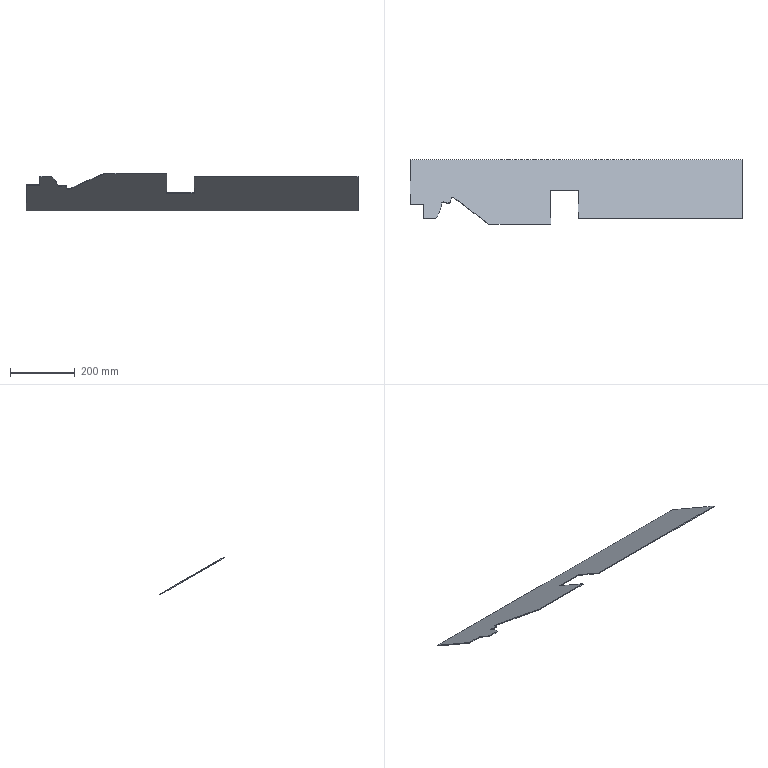Part | NX | features solid 2 | 1 solid | 15 faces | box 1023 x 199.923 x 116.58 mm | volume 412824 mm3 | plane 14 | spline 1
STEP:
#1=CARTESIAN_POINT('',(-459.422,185.,-80.));
#2=VERTEX_POINT('',#1);
#3=CARTESIAN_POINT('',(-459.422,186.,-78.268));
#4=VERTEX_POINT('',#3);
#5=CARTESIAN_POINT('',(-459.422,185.,-80.));
#6=DIRECTION('',(0.,0.5,0.866));
#7=VECTOR('',#6,1000.);
#8=LINE('',#5,#7);
#9=EDGE_CURVE('',#2,#4,#8,.T.);
#10=ORIENTED_EDGE('',*,*,#9,.T.);
#11=CARTESIAN_POINT('',(-502.5,186.,-78.268));
#12=VERTEX_POINT('',#11);
#13=CARTESIAN_POINT('',(255.,186.,-78.268));
#14=DIRECTION('',(1.,0.,0.));
#15=VECTOR('',#14,1000.);
#16=LINE('',#13,#15);
#17=EDGE_CURVE('',#12,#4,#16,.T.);
#18=ORIENTED_EDGE('',*,*,#17,.F.);
#19=CARTESIAN_POINT('',(-502.5,185.,-80.));
#20=VERTEX_POINT('',#19);
#21=CARTESIAN_POINT('',(-502.5,185.,-80.));
#22=DIRECTION('',(0.,0.5,0.866));
#23=VECTOR('',#22,1000.);
#24=LINE('',#21,#23);
#25=EDGE_CURVE('',#20,#12,#24,.T.);
#26=ORIENTED_EDGE('',*,*,#25,.F.);
#27=CARTESIAN_POINT('',(255.,185.,-80.));
#28=DIRECTION('',(-1.,0.,0.));
#29=VECTOR('',#28,1000.);
#30=LINE('',#27,#29);
#31=EDGE_CURVE('',#2,#20,#30,.T.);
#32=ORIENTED_EDGE('',*,*,#31,.F.);
#33=EDGE_LOOP('',(#10,#18,#26,#32));
#34=FACE_BOUND('',#33,.T.);
#35=CARTESIAN_POINT('',(255.,185.,-80.));
#36=DIRECTION('',(0.,0.866,-0.5));
#37=DIRECTION('',(0.,0.5,0.866));
#38=AXIS2_PLACEMENT_3D('',#35,#36,#37);
#39=PLANE('',#38);
#40=ADVANCED_FACE('',(#34),#39,.F.);
#41=CARTESIAN_POINT('',(-459.422,142.699,-53.268));
#42=VERTEX_POINT('',#41);
#43=CARTESIAN_POINT('',(-459.422,141.,-52.287));
#44=DIRECTION('',(0.,0.866,-0.5));
#45=VECTOR('',#44,1000.);
#46=LINE('',#43,#45);
#47=EDGE_CURVE('',#42,#4,#46,.T.);
#48=ORIENTED_EDGE('',*,*,#47,.T.);
#49=ORIENTED_EDGE('',*,*,#9,.F.);
#50=CARTESIAN_POINT('',(-459.422,141.699,-55.));
#51=VERTEX_POINT('',#50);
#52=CARTESIAN_POINT('',(-459.422,140.,-54.019));
#53=DIRECTION('',(0.,0.866,-0.5));
#54=VECTOR('',#53,1000.);
#55=LINE('',#52,#54);
#56=EDGE_CURVE('',#51,#2,#55,.T.);
#57=ORIENTED_EDGE('',*,*,#56,.F.);
#58=CARTESIAN_POINT('',(-459.422,141.699,-55.));
#59=DIRECTION('',(0.,0.5,0.866));
#60=VECTOR('',#59,1000.);
#61=LINE('',#58,#60);
#62=EDGE_CURVE('',#51,#42,#61,.T.);
#63=ORIENTED_EDGE('',*,*,#62,.T.);
#64=EDGE_LOOP('',(#48,#49,#57,#63));
#65=FACE_BOUND('',#64,.T.);
#66=CARTESIAN_POINT('',(-459.422,140.,-54.019));
#67=DIRECTION('',(1.,0.,0.));
#68=DIRECTION('',(0.,0.,-1.));
#69=AXIS2_PLACEMENT_3D('',#66,#67,#68);
#70=PLANE('',#69);
#71=ADVANCED_FACE('',(#65),#70,.F.);
#72=CARTESIAN_POINT('',(-425.175,142.699,-53.268));
#73=VERTEX_POINT('',#72);
#74=CARTESIAN_POINT('',(-690.,142.699,-53.268));
#75=DIRECTION('',(1.,0.,0.));
#76=VECTOR('',#75,1000.);
#77=LINE('',#74,#76);
#78=EDGE_CURVE('',#42,#73,#77,.T.);
#79=ORIENTED_EDGE('',*,*,#78,.F.);
#80=ORIENTED_EDGE('',*,*,#62,.F.);
#81=CARTESIAN_POINT('',(-425.175,141.699,-55.));
#82=VERTEX_POINT('',#81);
#83=CARTESIAN_POINT('',(-690.,141.699,-55.));
#84=DIRECTION('',(1.,0.,0.));
#85=VECTOR('',#84,1000.);
#86=LINE('',#83,#85);
#87=EDGE_CURVE('',#51,#82,#86,.T.);
#88=ORIENTED_EDGE('',*,*,#87,.T.);
#89=CARTESIAN_POINT('',(-425.175,142.199,-54.134));
#90=DIRECTION('',(0.,0.5,0.866));
#91=VECTOR('',#90,1000.);
#92=LINE('',#89,#91);
#93=EDGE_CURVE('',#82,#73,#92,.T.);
#94=ORIENTED_EDGE('',*,*,#93,.T.);
#95=EDGE_LOOP('',(#79,#80,#88,#94));
#96=FACE_BOUND('',#95,.T.);
#97=CARTESIAN_POINT('',(-690.,141.699,-55.));
#98=DIRECTION('',(0.,-0.866,0.5));
#99=DIRECTION('',(0.,-0.5,-0.866));
#100=AXIS2_PLACEMENT_3D('',#97,#98,#99);
#101=PLANE('',#100);
#102=ADVANCED_FACE('',(#96),#101,.T.);
#103=CARTESIAN_POINT('',(-302.263,157.613,-61.879));
#104=VERTEX_POINT('',#103);
#105=CARTESIAN_POINT('',(-425.175,142.699,-53.268));
#106=CARTESIAN_POINT('',(-423.944,144.129,-54.094));
#107=CARTESIAN_POINT('',(-422.094,146.273,-55.331));
#108=CARTESIAN_POINT('',(-419.64,149.138,-56.986));
#109=CARTESIAN_POINT('',(-417.767,151.269,-58.216));
#110=CARTESIAN_POINT('',(-416.02,153.47,-59.487));
#111=CARTESIAN_POINT('',(-414.143,156.651,-61.323));
#112=CARTESIAN_POINT('',(-412.51,161.038,-63.856));
#113=CARTESIAN_POINT('',(-411.153,166.385,-66.943));
#114=CARTESIAN_POINT('',(-409.846,171.751,-70.041));
#115=CARTESIAN_POINT('',(-408.496,177.106,-73.133));
#116=CARTESIAN_POINT('',(-407.476,181.591,-75.723));
#117=CARTESIAN_POINT('',(-406.489,185.141,-77.772));
#118=CARTESIAN_POINT('',(-405.589,187.771,-79.29));
#119=CARTESIAN_POINT('',(-404.452,190.331,-80.768));
#120=CARTESIAN_POINT('',(-402.998,192.277,-81.892));
#121=CARTESIAN_POINT('',(-401.24,193.353,-82.513));
#122=CARTESIAN_POINT('',(-399.144,193.752,-82.744));
#123=CARTESIAN_POINT('',(-396.529,193.151,-82.397));
#124=CARTESIAN_POINT('',(-393.666,192.058,-81.766));
#125=CARTESIAN_POINT('',(-390.775,190.954,-81.128));
#126=CARTESIAN_POINT('',(-387.755,190.191,-80.687));
#127=CARTESIAN_POINT('',(-384.597,190.018,-80.588));
#128=CARTESIAN_POINT('',(-381.485,190.907,-81.101));
#129=CARTESIAN_POINT('',(-379.542,193.151,-82.397));
#130=CARTESIAN_POINT('',(-378.509,195.729,-83.885));
#131=CARTESIAN_POINT('',(-377.875,198.386,-85.419));
#132=CARTESIAN_POINT('',(-377.182,201.03,-86.945));
#133=CARTESIAN_POINT('',(-376.325,203.647,-88.457));
#134=CARTESIAN_POINT('',(-375.054,206.119,-89.884));
#135=CARTESIAN_POINT('',(-373.395,207.96,-90.947));
#136=CARTESIAN_POINT('',(-371.441,208.706,-91.377));
#137=CARTESIAN_POINT('',(-369.836,208.668,-91.355));
#138=CARTESIAN_POINT('',(-368.391,208.101,-91.028));
#139=CARTESIAN_POINT('',(-366.706,207.022,-90.405));
#140=CARTESIAN_POINT('',(-364.874,205.442,-89.493));
#141=CARTESIAN_POINT('',(-362.118,202.752,-87.94));
#142=CARTESIAN_POINT('',(-358.537,199.522,-86.075));
#143=CARTESIAN_POINT('',(-353.538,196.335,-84.235));
#144=CARTESIAN_POINT('',(-348.779,192.912,-82.259));
#145=CARTESIAN_POINT('',(-344.265,189.246,-80.142));
#146=CARTESIAN_POINT('',(-339.632,185.697,-78.093));
#147=CARTESIAN_POINT('',(-334.916,182.231,-76.092));
#148=CARTESIAN_POINT('',(-328.709,177.53,-73.378));
#149=CARTESIAN_POINT('',(-320.935,171.667,-69.993));
#150=CARTESIAN_POINT('',(-311.588,164.651,-65.942));
#151=CARTESIAN_POINT('',(-305.369,159.962,-63.235));
#152=CARTESIAN_POINT('',(-302.263,157.613,-61.879));
#153=B_SPLINE_CURVE_WITH_KNOTS('',3,(#105,#106,#107,#108,#109,#110,#111,#112,#113,#114,#115,#116,#117,#118,#119,#120,#121,#122,#123,#124,#125,#126,#127,#128,#129,#130,#131,#132,#133,#134,#135,#136,#137,#138,#139,#140,#141,#142,#143,#144,#145,#146,#147,#148,#149,#150,#151,#152),.UNSPECIFIED.,.F.,.F.,(4,1,1,1,1,1,1,1,1,1,1,1,1,1,1,1,1,1,1,1,1,1,1,1,1,1,1,1,1,1,1,1,1,1,1,1,1,1,1,1,1,1,1,1,1,4),(0.,0.006163,0.009244,0.01233,0.01541,0.01849,0.02465,0.03081,0.03698,0.04314,0.0493,0.05239,0.05547,0.05855,0.06163,0.06317,0.06471,0.06779,0.07087,0.07396,0.07704,0.08012,0.0832,0.08628,0.08936,0.09244,0.09553,0.09861,0.1017,0.1048,0.1063,0.1079,0.1094,0.1109,0.114,0.1171,0.1233,0.1294,0.1356,0.1417,0.1479,0.1541,0.1602,0.1726,0.1849,0.1972),.UNSPECIFIED.);
#154=EDGE_CURVE('',#73,#104,#153,.T.);
#155=ORIENTED_EDGE('',*,*,#154,.F.);
#156=ORIENTED_EDGE('',*,*,#93,.F.);
#157=CARTESIAN_POINT('',(-302.263,156.613,-63.611));
#158=VERTEX_POINT('',#157);
#159=CARTESIAN_POINT('',(-425.175,141.699,-55.));
#160=CARTESIAN_POINT('',(-423.944,143.129,-55.826));
#161=CARTESIAN_POINT('',(-422.094,145.273,-57.064));
#162=CARTESIAN_POINT('',(-419.64,148.138,-58.718));
#163=CARTESIAN_POINT('',(-417.767,150.269,-59.948));
#164=CARTESIAN_POINT('',(-416.02,152.47,-61.219));
#165=CARTESIAN_POINT('',(-414.143,155.651,-63.055));
#166=CARTESIAN_POINT('',(-412.51,160.038,-65.588));
#167=CARTESIAN_POINT('',(-411.153,165.385,-68.675));
#168=CARTESIAN_POINT('',(-409.846,170.751,-71.774));
#169=CARTESIAN_POINT('',(-408.496,176.106,-74.865));
#170=CARTESIAN_POINT('',(-407.476,180.591,-77.455));
#171=CARTESIAN_POINT('',(-406.489,184.141,-79.504));
#172=CARTESIAN_POINT('',(-405.589,186.771,-81.022));
#173=CARTESIAN_POINT('',(-404.452,189.331,-82.5));
#174=CARTESIAN_POINT('',(-402.998,191.277,-83.624));
#175=CARTESIAN_POINT('',(-401.24,192.353,-84.245));
#176=CARTESIAN_POINT('',(-399.144,192.752,-84.476));
#177=CARTESIAN_POINT('',(-396.529,192.151,-84.129));
#178=CARTESIAN_POINT('',(-393.666,191.058,-83.498));
#179=CARTESIAN_POINT('',(-390.775,189.954,-82.86));
#180=CARTESIAN_POINT('',(-387.755,189.191,-82.419));
#181=CARTESIAN_POINT('',(-384.597,189.018,-82.32));
#182=CARTESIAN_POINT('',(-381.485,189.907,-82.833));
#183=CARTESIAN_POINT('',(-379.542,192.151,-84.129));
#184=CARTESIAN_POINT('',(-378.509,194.729,-85.617));
#185=CARTESIAN_POINT('',(-377.875,197.386,-87.151));
#186=CARTESIAN_POINT('',(-377.182,200.03,-88.678));
#187=CARTESIAN_POINT('',(-376.325,202.647,-90.189));
#188=CARTESIAN_POINT('',(-375.054,205.119,-91.616));
#189=CARTESIAN_POINT('',(-373.395,206.96,-92.679));
#190=CARTESIAN_POINT('',(-371.441,207.706,-93.109));
#191=CARTESIAN_POINT('',(-369.836,207.668,-93.087));
#192=CARTESIAN_POINT('',(-368.391,207.101,-92.76));
#193=CARTESIAN_POINT('',(-366.706,206.022,-92.137));
#194=CARTESIAN_POINT('',(-364.874,204.442,-91.225));
#195=CARTESIAN_POINT('',(-362.118,201.752,-89.672));
#196=CARTESIAN_POINT('',(-358.537,198.522,-87.807));
#197=CARTESIAN_POINT('',(-353.538,195.335,-85.967));
#198=CARTESIAN_POINT('',(-348.779,191.912,-83.991));
#199=CARTESIAN_POINT('',(-344.265,188.246,-81.874));
#200=CARTESIAN_POINT('',(-339.632,184.697,-79.825));
#201=CARTESIAN_POINT('',(-334.916,181.231,-77.824));
#202=CARTESIAN_POINT('',(-328.709,176.53,-75.11));
#203=CARTESIAN_POINT('',(-320.935,170.667,-71.725));
#204=CARTESIAN_POINT('',(-311.588,163.651,-67.674));
#205=CARTESIAN_POINT('',(-305.369,158.962,-64.967));
#206=CARTESIAN_POINT('',(-302.263,156.613,-63.611));
#207=B_SPLINE_CURVE_WITH_KNOTS('',3,(#159,#160,#161,#162,#163,#164,#165,#166,#167,#168,#169,#170,#171,#172,#173,#174,#175,#176,#177,#178,#179,#180,#181,#182,#183,#184,#185,#186,#187,#188,#189,#190,#191,#192,#193,#194,#195,#196,#197,#198,#199,#200,#201,#202,#203,#204,#205,#206),.UNSPECIFIED.,.F.,.F.,(4,1,1,1,1,1,1,1,1,1,1,1,1,1,1,1,1,1,1,1,1,1,1,1,1,1,1,1,1,1,1,1,1,1,1,1,1,1,1,1,1,1,1,1,1,4),(0.,0.006163,0.009244,0.01233,0.01541,0.01849,0.02465,0.03081,0.03698,0.04314,0.0493,0.05239,0.05547,0.05855,0.06163,0.06317,0.06471,0.06779,0.07087,0.07396,0.07704,0.08012,0.0832,0.08628,0.08936,0.09244,0.09553,0.09861,0.1017,0.1048,0.1063,0.1079,0.1094,0.1109,0.114,0.1171,0.1233,0.1294,0.1356,0.1417,0.1479,0.1541,0.1602,0.1726,0.1849,0.1972),.UNSPECIFIED.);
#208=EDGE_CURVE('',#82,#158,#207,.T.);
#209=ORIENTED_EDGE('',*,*,#208,.T.);
#210=CARTESIAN_POINT('',(-302.263,156.613,-63.611));
#211=CARTESIAN_POINT('',(-302.263,156.946,-63.033));
#212=CARTESIAN_POINT('',(-302.263,157.28,-62.456));
#213=CARTESIAN_POINT('',(-302.263,157.613,-61.879));
#214=B_SPLINE_CURVE_WITH_KNOTS('',3,(#210,#211,#212,#213),.UNSPECIFIED.,.F.,.F.,(4,4),(0.,1.),.UNSPECIFIED.);
#215=EDGE_CURVE('',#158,#104,#214,.T.);
#216=ORIENTED_EDGE('',*,*,#215,.T.);
#217=EDGE_LOOP('',(#155,#156,#209,#216));
#218=FACE_BOUND('',#217,.T.);
#219=CARTESIAN_POINT('',(-425.175,141.699,-55.));
#220=CARTESIAN_POINT('',(-425.175,142.699,-53.268));
#221=CARTESIAN_POINT('',(-423.93,143.145,-55.835));
#222=CARTESIAN_POINT('',(-423.93,144.145,-54.103));
#223=CARTESIAN_POINT('',(-422.059,145.312,-57.086));
#224=CARTESIAN_POINT('',(-422.059,146.312,-55.354));
#225=CARTESIAN_POINT('',(-419.581,148.209,-58.759));
#226=CARTESIAN_POINT('',(-419.581,149.209,-57.027));
#227=CARTESIAN_POINT('',(-417.68,150.364,-60.003));
#228=CARTESIAN_POINT('',(-417.68,151.364,-58.271));
#229=CARTESIAN_POINT('',(-416.23,152.215,-61.072));
#230=CARTESIAN_POINT('',(-416.23,153.215,-59.339));
#231=CARTESIAN_POINT('',(-415.245,153.789,-61.98));
#232=CARTESIAN_POINT('',(-415.245,154.789,-60.248));
#233=CARTESIAN_POINT('',(-414.6,154.974,-62.665));
#234=CARTESIAN_POINT('',(-414.6,155.974,-60.933));
#235=CARTESIAN_POINT('',(-414.081,156.071,-63.298));
#236=CARTESIAN_POINT('',(-414.081,157.071,-61.566));
#237=CARTESIAN_POINT('',(-413.551,157.337,-64.029));
#238=CARTESIAN_POINT('',(-413.551,158.337,-62.297));
#239=CARTESIAN_POINT('',(-413.148,158.42,-64.654));
#240=CARTESIAN_POINT('',(-413.148,159.42,-62.922));
#241=CARTESIAN_POINT('',(-412.803,159.445,-65.246));
#242=CARTESIAN_POINT('',(-412.803,160.445,-63.514));
#243=CARTESIAN_POINT('',(-412.599,160.082,-65.613));
#244=CARTESIAN_POINT('',(-412.599,161.082,-63.881));
#245=CARTESIAN_POINT('',(-412.286,161.116,-66.211));
#246=CARTESIAN_POINT('',(-412.286,162.116,-64.479));
#247=CARTESIAN_POINT('',(-411.922,162.416,-66.961));
#248=CARTESIAN_POINT('',(-411.922,163.416,-65.229));
#249=CARTESIAN_POINT('',(-411.59,163.68,-67.691));
#250=CARTESIAN_POINT('',(-411.59,164.68,-65.959));
#251=CARTESIAN_POINT('',(-411.348,164.644,-68.247));
#252=CARTESIAN_POINT('',(-411.348,165.644,-66.515));
#253=CARTESIAN_POINT('',(-411.133,165.499,-68.741));
#254=CARTESIAN_POINT('',(-411.133,166.499,-67.009));
#255=CARTESIAN_POINT('',(-410.857,166.606,-69.38));
#256=CARTESIAN_POINT('',(-410.857,167.606,-67.648));
#257=CARTESIAN_POINT('',(-410.424,168.356,-70.391));
#258=CARTESIAN_POINT('',(-410.424,169.356,-68.659));
#259=CARTESIAN_POINT('',(-409.996,170.117,-71.407));
#260=CARTESIAN_POINT('',(-409.996,171.117,-69.675));
#261=CARTESIAN_POINT('',(-409.563,171.864,-72.416));
#262=CARTESIAN_POINT('',(-409.563,172.864,-70.684));
#263=CARTESIAN_POINT('',(-409.283,172.979,-73.06));
#264=CARTESIAN_POINT('',(-409.283,173.979,-71.328));
#265=CARTESIAN_POINT('',(-409.099,173.712,-73.483));
#266=CARTESIAN_POINT('',(-409.099,174.712,-71.751));
#267=CARTESIAN_POINT('',(-408.973,174.205,-73.768));
#268=CARTESIAN_POINT('',(-408.973,175.205,-72.036));
#269=CARTESIAN_POINT('',(-408.94,174.342,-73.847));
#270=CARTESIAN_POINT('',(-408.94,175.342,-72.114));
#271=CARTESIAN_POINT('',(-408.83,174.79,-74.105));
#272=CARTESIAN_POINT('',(-408.83,175.79,-72.373));
#273=CARTESIAN_POINT('',(-408.62,175.675,-74.616));
#274=CARTESIAN_POINT('',(-408.62,176.675,-72.884));
#275=CARTESIAN_POINT('',(-408.278,177.127,-75.454));
#276=CARTESIAN_POINT('',(-408.278,178.127,-73.722));
#277=CARTESIAN_POINT('',(-408.039,178.144,-76.042));
#278=CARTESIAN_POINT('',(-408.039,179.144,-74.31));
#279=CARTESIAN_POINT('',(-407.925,178.624,-76.319));
#280=CARTESIAN_POINT('',(-407.925,179.624,-74.587));
#281=CARTESIAN_POINT('',(-407.848,178.947,-76.505));
#282=CARTESIAN_POINT('',(-407.848,179.947,-74.773));
#283=CARTESIAN_POINT('',(-407.821,179.059,-76.57));
#284=CARTESIAN_POINT('',(-407.821,180.059,-74.838));
#285=CARTESIAN_POINT('',(-407.71,179.52,-76.836));
#286=CARTESIAN_POINT('',(-407.71,180.52,-75.104));
#287=CARTESIAN_POINT('',(-407.592,179.999,-77.112));
#288=CARTESIAN_POINT('',(-407.592,180.999,-75.38));
#289=CARTESIAN_POINT('',(-407.437,180.619,-77.47));
#290=CARTESIAN_POINT('',(-407.437,181.619,-75.738));
#291=CARTESIAN_POINT('',(-407.2,181.542,-78.003));
#292=CARTESIAN_POINT('',(-407.2,182.542,-76.271));
#293=CARTESIAN_POINT('',(-406.966,182.408,-78.503));
#294=CARTESIAN_POINT('',(-406.966,183.408,-76.771));
#295=CARTESIAN_POINT('',(-406.744,183.193,-78.957));
#296=CARTESIAN_POINT('',(-406.744,184.193,-77.225));
#297=CARTESIAN_POINT('',(-406.601,183.681,-79.239));
#298=CARTESIAN_POINT('',(-406.601,184.681,-77.507));
#299=CARTESIAN_POINT('',(-406.505,183.998,-79.422));
#300=CARTESIAN_POINT('',(-406.505,184.998,-77.69));
#301=CARTESIAN_POINT('',(-406.332,184.556,-79.744));
#302=CARTESIAN_POINT('',(-406.332,185.556,-78.012));
#303=CARTESIAN_POINT('',(-406.062,185.383,-80.221));
#304=CARTESIAN_POINT('',(-406.062,186.383,-78.489));
#305=CARTESIAN_POINT('',(-405.65,186.534,-80.886));
#306=CARTESIAN_POINT('',(-405.65,187.534,-79.154));
#307=CARTESIAN_POINT('',(-405.229,187.547,-81.471));
#308=CARTESIAN_POINT('',(-405.229,188.547,-79.739));
#309=CARTESIAN_POINT('',(-404.934,188.186,-81.839));
#310=CARTESIAN_POINT('',(-404.934,189.186,-80.107));
#311=CARTESIAN_POINT('',(-404.754,188.55,-82.05));
#312=CARTESIAN_POINT('',(-404.754,189.55,-80.318));
#313=CARTESIAN_POINT('',(-404.645,188.764,-82.173));
#314=CARTESIAN_POINT('',(-404.645,189.764,-80.441));
#315=CARTESIAN_POINT('',(-404.409,189.199,-82.425));
#316=CARTESIAN_POINT('',(-404.409,190.199,-80.692));
#317=CARTESIAN_POINT('',(-404.128,189.668,-82.695));
#318=CARTESIAN_POINT('',(-404.128,190.668,-80.963));
#319=CARTESIAN_POINT('',(-403.592,190.455,-83.15));
#320=CARTESIAN_POINT('',(-403.592,191.455,-81.418));
#321=CARTESIAN_POINT('',(-402.773,191.355,-83.669));
#322=CARTESIAN_POINT('',(-402.773,192.355,-81.937));
#323=CARTESIAN_POINT('',(-401.67,192.113,-84.106));
#324=CARTESIAN_POINT('',(-401.67,193.113,-82.374));
#325=CARTESIAN_POINT('',(-400.497,192.552,-84.36));
#326=CARTESIAN_POINT('',(-400.497,193.552,-82.628));
#327=CARTESIAN_POINT('',(-399.224,192.615,-84.396));
#328=CARTESIAN_POINT('',(-399.224,193.615,-82.664));
#329=CARTESIAN_POINT('',(-398.324,192.504,-84.332));
#330=CARTESIAN_POINT('',(-398.324,193.504,-82.6));
#331=CARTESIAN_POINT('',(-397.844,192.414,-84.28));
#332=CARTESIAN_POINT('',(-397.844,193.414,-82.548));
#333=CARTESIAN_POINT('',(-397.672,192.378,-84.26));
#334=CARTESIAN_POINT('',(-397.672,193.378,-82.528));
#335=CARTESIAN_POINT('',(-397.283,192.29,-84.209));
#336=CARTESIAN_POINT('',(-397.283,193.29,-82.477));
#337=CARTESIAN_POINT('',(-396.713,192.135,-84.119));
#338=CARTESIAN_POINT('',(-396.713,193.135,-82.387));
#339=CARTESIAN_POINT('',(-395.957,191.899,-83.983));
#340=CARTESIAN_POINT('',(-395.957,192.899,-82.251));
#341=CARTESIAN_POINT('',(-395.051,191.576,-83.796));
#342=CARTESIAN_POINT('',(-395.051,192.576,-82.064));
#343=CARTESIAN_POINT('',(-394.15,191.239,-83.602));
#344=CARTESIAN_POINT('',(-394.15,192.239,-81.87));
#345=CARTESIAN_POINT('',(-392.918,190.777,-83.335));
#346=CARTESIAN_POINT('',(-392.918,191.777,-81.603));
#347=CARTESIAN_POINT('',(-391.508,190.238,-83.024));
#348=CARTESIAN_POINT('',(-391.508,191.238,-81.292));
#349=CARTESIAN_POINT('',(-390.066,189.791,-82.766));
#350=CARTESIAN_POINT('',(-390.066,190.791,-81.034));
#351=CARTESIAN_POINT('',(-388.325,189.358,-82.516));
#352=CARTESIAN_POINT('',(-388.325,190.358,-80.784));
#353=CARTESIAN_POINT('',(-386.714,189.142,-82.391));
#354=CARTESIAN_POINT('',(-386.714,190.142,-80.659));
#355=CARTESIAN_POINT('',(-385.47,189.115,-82.376));
#356=CARTESIAN_POINT('',(-385.47,190.115,-80.644));
#357=CARTESIAN_POINT('',(-384.509,189.199,-82.424));
#358=CARTESIAN_POINT('',(-384.509,190.199,-80.692));
#359=CARTESIAN_POINT('',(-383.876,189.293,-82.479));
#360=CARTESIAN_POINT('',(-383.876,190.293,-80.747));
#361=CARTESIAN_POINT('',(-383.025,189.503,-82.6));
#362=CARTESIAN_POINT('',(-383.025,190.503,-80.868));
#363=CARTESIAN_POINT('',(-382.083,189.865,-82.809));
#364=CARTESIAN_POINT('',(-382.083,190.865,-81.077));
#365=CARTESIAN_POINT('',(-381.055,190.511,-83.182));
#366=CARTESIAN_POINT('',(-381.055,191.511,-81.45));
#367=CARTESIAN_POINT('',(-380.28,191.34,-83.66));
#368=CARTESIAN_POINT('',(-380.28,192.34,-81.928));
#369=CARTESIAN_POINT('',(-379.791,192.037,-84.063));
#370=CARTESIAN_POINT('',(-379.791,193.037,-82.331));
#371=CARTESIAN_POINT('',(-379.514,192.508,-84.335));
#372=CARTESIAN_POINT('',(-379.514,193.508,-82.603));
#373=CARTESIAN_POINT('',(-379.334,192.843,-84.528));
#374=CARTESIAN_POINT('',(-379.334,193.843,-82.796));
#375=CARTESIAN_POINT('',(-379.091,193.347,-84.819));
#376=CARTESIAN_POINT('',(-379.091,194.347,-83.087));
#377=CARTESIAN_POINT('',(-378.828,193.996,-85.194));
#378=CARTESIAN_POINT('',(-378.828,194.996,-83.462));
#379=CARTESIAN_POINT('',(-378.652,194.498,-85.484));
#380=CARTESIAN_POINT('',(-378.652,195.498,-83.751));
#381=CARTESIAN_POINT('',(-378.527,194.897,-85.714));
#382=CARTESIAN_POINT('',(-378.527,195.897,-83.982));
#383=CARTESIAN_POINT('',(-378.494,195.007,-85.778));
#384=CARTESIAN_POINT('',(-378.494,196.007,-84.046));
#385=CARTESIAN_POINT('',(-378.406,195.306,-85.95));
#386=CARTESIAN_POINT('',(-378.406,196.306,-84.218));
#387=CARTESIAN_POINT('',(-378.276,195.779,-86.223));
#388=CARTESIAN_POINT('',(-378.276,196.779,-84.491));
#389=CARTESIAN_POINT('',(-378.09,196.484,-86.63));
#390=CARTESIAN_POINT('',(-378.09,197.484,-84.898));
#391=CARTESIAN_POINT('',(-377.869,197.369,-87.141));
#392=CARTESIAN_POINT('',(-377.869,198.369,-85.409));
#393=CARTESIAN_POINT('',(-377.593,198.467,-87.775));
#394=CARTESIAN_POINT('',(-377.593,199.467,-86.043));
#395=CARTESIAN_POINT('',(-377.254,199.71,-88.493));
#396=CARTESIAN_POINT('',(-377.254,200.71,-86.761));
#397=CARTESIAN_POINT('',(-376.928,200.782,-89.112));
#398=CARTESIAN_POINT('',(-376.928,201.782,-87.38));
#399=CARTESIAN_POINT('',(-376.682,201.517,-89.536));
#400=CARTESIAN_POINT('',(-376.682,202.517,-87.804));
#401=CARTESIAN_POINT('',(-376.516,201.97,-89.798));
#402=CARTESIAN_POINT('',(-376.516,202.97,-88.066));
#403=CARTESIAN_POINT('',(-376.421,202.22,-89.942));
#404=CARTESIAN_POINT('',(-376.421,203.22,-88.21));
#405=CARTESIAN_POINT('',(-376.181,202.81,-90.283));
#406=CARTESIAN_POINT('',(-376.181,203.81,-88.551));
#407=CARTESIAN_POINT('',(-375.81,203.626,-90.754));
#408=CARTESIAN_POINT('',(-375.81,204.626,-89.022));
#409=CARTESIAN_POINT('',(-375.196,204.74,-91.397));
#410=CARTESIAN_POINT('',(-375.196,205.74,-89.665));
#411=CARTESIAN_POINT('',(-374.545,205.625,-91.908));
#412=CARTESIAN_POINT('',(-374.545,206.625,-90.176));
#413=CARTESIAN_POINT('',(-373.956,206.246,-92.266));
#414=CARTESIAN_POINT('',(-373.956,207.246,-90.534));
#415=CARTESIAN_POINT('',(-373.573,206.602,-92.472));
#416=CARTESIAN_POINT('',(-373.573,207.602,-90.74));
#417=CARTESIAN_POINT('',(-372.86,207.112,-92.766));
#418=CARTESIAN_POINT('',(-372.86,208.112,-91.034));
#419=CARTESIAN_POINT('',(-371.968,207.524,-93.004));
#420=CARTESIAN_POINT('',(-371.968,208.524,-91.272));
#421=CARTESIAN_POINT('',(-370.705,207.759,-93.14));
#422=CARTESIAN_POINT('',(-370.705,208.759,-91.408));
#423=CARTESIAN_POINT('',(-369.525,207.538,-93.012));
#424=CARTESIAN_POINT('',(-369.525,208.538,-91.28));
#425=CARTESIAN_POINT('',(-368.664,207.191,-92.812));
#426=CARTESIAN_POINT('',(-368.664,208.191,-91.08));
#427=CARTESIAN_POINT('',(-368.1,206.892,-92.639));
#428=CARTESIAN_POINT('',(-368.1,207.892,-90.907));
#429=CARTESIAN_POINT('',(-367.794,206.71,-92.534));
#430=CARTESIAN_POINT('',(-367.794,207.71,-90.802));
#431=CARTESIAN_POINT('',(-367.295,206.39,-92.349));
#432=CARTESIAN_POINT('',(-367.295,207.39,-90.617));
#433=CARTESIAN_POINT('',(-366.687,205.945,-92.093));
#434=CARTESIAN_POINT('',(-366.687,206.945,-90.36));
#435=CARTESIAN_POINT('',(-366.22,205.574,-91.879));
#436=CARTESIAN_POINT('',(-366.22,206.574,-90.147));
#437=CARTESIAN_POINT('',(-365.855,205.27,-91.703));
#438=CARTESIAN_POINT('',(-365.855,206.27,-89.971));
#439=CARTESIAN_POINT('',(-365.736,205.168,-91.644));
#440=CARTESIAN_POINT('',(-365.736,206.168,-89.912));
#441=CARTESIAN_POINT('',(-365.296,204.79,-91.425));
#442=CARTESIAN_POINT('',(-365.296,205.79,-89.693));
#443=CARTESIAN_POINT('',(-364.659,204.208,-91.09));
#444=CARTESIAN_POINT('',(-364.659,205.208,-89.358));
#445=CARTESIAN_POINT('',(-363.998,203.581,-90.728));
#446=CARTESIAN_POINT('',(-363.998,204.581,-88.996));
#447=CARTESIAN_POINT('',(-363.434,203.04,-90.416));
#448=CARTESIAN_POINT('',(-363.434,204.04,-88.684));
#449=CARTESIAN_POINT('',(-362.971,202.598,-90.16));
#450=CARTESIAN_POINT('',(-362.971,203.598,-88.428));
#451=CARTESIAN_POINT('',(-362.474,202.124,-89.887));
#452=CARTESIAN_POINT('',(-362.474,203.124,-88.155));
#453=CARTESIAN_POINT('',(-362.133,201.8,-89.7));
#454=CARTESIAN_POINT('',(-362.133,202.8,-87.968));
#455=CARTESIAN_POINT('',(-361.937,201.616,-89.593));
#456=CARTESIAN_POINT('',(-361.937,202.616,-87.861));
#457=CARTESIAN_POINT('',(-361.888,201.57,-89.567));
#458=CARTESIAN_POINT('',(-361.888,202.57,-87.835));
#459=CARTESIAN_POINT('',(-361.655,201.353,-89.442));
#460=CARTESIAN_POINT('',(-361.655,202.353,-87.709));
#461=CARTESIAN_POINT('',(-361.43,201.147,-89.323));
#462=CARTESIAN_POINT('',(-361.43,202.147,-87.591));
#463=CARTESIAN_POINT('',(-360.852,200.623,-89.02));
#464=CARTESIAN_POINT('',(-360.852,201.623,-87.288));
#465=CARTESIAN_POINT('',(-360.051,199.924,-88.617));
#466=CARTESIAN_POINT('',(-360.051,200.924,-86.884));
#467=CARTESIAN_POINT('',(-359.078,199.134,-88.16));
#468=CARTESIAN_POINT('',(-359.078,200.134,-86.428));
#469=CARTESIAN_POINT('',(-357.95,198.278,-87.666));
#470=CARTESIAN_POINT('',(-357.95,199.278,-85.934));
#471=CARTESIAN_POINT('',(-356.922,197.543,-87.242));
#472=CARTESIAN_POINT('',(-356.922,198.543,-85.51));
#473=CARTESIAN_POINT('',(-356.143,197.007,-86.932));
#474=CARTESIAN_POINT('',(-356.143,198.007,-85.2));
#475=CARTESIAN_POINT('',(-355.749,196.741,-86.778));
#476=CARTESIAN_POINT('',(-355.749,197.741,-85.046));
#477=CARTESIAN_POINT('',(-355.507,196.578,-86.685));
#478=CARTESIAN_POINT('',(-355.507,197.578,-84.953));
#479=CARTESIAN_POINT('',(-355.36,196.481,-86.628));
#480=CARTESIAN_POINT('',(-355.36,197.481,-84.896));
#481=CARTESIAN_POINT('',(-355.042,196.269,-86.506));
#482=CARTESIAN_POINT('',(-355.042,197.269,-84.774));
#483=CARTESIAN_POINT('',(-354.706,196.046,-86.378));
#484=CARTESIAN_POINT('',(-354.706,197.046,-84.646));
#485=CARTESIAN_POINT('',(-354.152,195.678,-86.165));
#486=CARTESIAN_POINT('',(-354.152,196.678,-84.433));
#487=CARTESIAN_POINT('',(-353.548,195.277,-85.933));
#488=CARTESIAN_POINT('',(-353.548,196.277,-84.201));
#489=CARTESIAN_POINT('',(-353.197,195.043,-85.798));
#490=CARTESIAN_POINT('',(-353.197,196.043,-84.066));
#491=CARTESIAN_POINT('',(-353.036,194.935,-85.736));
#492=CARTESIAN_POINT('',(-353.036,195.935,-84.004));
#493=CARTESIAN_POINT('',(-353.043,194.939,-85.739));
#494=CARTESIAN_POINT('',(-353.043,195.939,-84.007));
#495=CARTESIAN_POINT('',(-352.792,194.769,-85.64));
#496=CARTESIAN_POINT('',(-352.792,195.769,-83.908));
#497=CARTESIAN_POINT('',(-352.567,194.614,-85.55));
#498=CARTESIAN_POINT('',(-352.567,195.614,-83.818));
#499=CARTESIAN_POINT('',(-352.156,194.329,-85.386));
#500=CARTESIAN_POINT('',(-352.156,195.329,-83.654));
#501=CARTESIAN_POINT('',(-351.652,193.974,-85.181));
#502=CARTESIAN_POINT('',(-351.652,194.974,-83.449));
#503=CARTESIAN_POINT('',(-351.157,193.619,-84.976));
#504=CARTESIAN_POINT('',(-351.157,194.619,-83.244));
#505=CARTESIAN_POINT('',(-350.722,193.303,-84.794));
#506=CARTESIAN_POINT('',(-350.722,194.303,-83.062));
#507=CARTESIAN_POINT('',(-350.294,192.988,-84.612));
#508=CARTESIAN_POINT('',(-350.294,193.988,-82.88));
#509=CARTESIAN_POINT('',(-349.489,192.387,-84.265));
#510=CARTESIAN_POINT('',(-349.489,193.387,-82.533));
#511=CARTESIAN_POINT('',(-348.359,191.519,-83.764));
#512=CARTESIAN_POINT('',(-348.359,192.519,-82.032));
#513=CARTESIAN_POINT('',(-347.263,190.661,-83.268));
#514=CARTESIAN_POINT('',(-347.263,191.661,-81.536));
#515=CARTESIAN_POINT('',(-346.405,189.98,-82.875));
#516=CARTESIAN_POINT('',(-346.405,190.98,-81.143));
#517=CARTESIAN_POINT('',(-345.203,189.024,-82.323));
#518=CARTESIAN_POINT('',(-345.203,190.024,-80.591));
#519=CARTESIAN_POINT('',(-344.051,188.111,-81.796));
#520=CARTESIAN_POINT('',(-344.051,189.111,-80.064));
#521=CARTESIAN_POINT('',(-342.935,187.231,-81.288));
#522=CARTESIAN_POINT('',(-342.935,188.231,-79.556));
#523=CARTESIAN_POINT('',(-342.313,186.747,-81.008));
#524=CARTESIAN_POINT('',(-342.313,187.747,-79.276));
#525=CARTESIAN_POINT('',(-342.053,186.547,-80.893));
#526=CARTESIAN_POINT('',(-342.053,187.547,-79.161));
#527=CARTESIAN_POINT('',(-341.761,186.323,-80.764));
#528=CARTESIAN_POINT('',(-341.761,187.323,-79.032));
#529=CARTESIAN_POINT('',(-341.251,185.936,-80.54));
#530=CARTESIAN_POINT('',(-341.251,186.936,-78.808));
#531=CARTESIAN_POINT('',(-340.366,185.269,-80.155));
#532=CARTESIAN_POINT('',(-340.366,186.269,-78.423));
#533=CARTESIAN_POINT('',(-339.326,184.492,-79.707));
#534=CARTESIAN_POINT('',(-339.326,185.492,-77.975));
#535=CARTESIAN_POINT('',(-338.486,183.869,-79.347));
#536=CARTESIAN_POINT('',(-338.486,184.869,-77.615));
#537=CARTESIAN_POINT('',(-338.009,183.516,-79.143));
#538=CARTESIAN_POINT('',(-338.009,184.516,-77.411));
#539=CARTESIAN_POINT('',(-337.556,183.181,-78.95));
#540=CARTESIAN_POINT('',(-337.556,184.181,-77.217));
#541=CARTESIAN_POINT('',(-337.424,183.083,-78.893));
#542=CARTESIAN_POINT('',(-337.424,184.083,-77.161));
#543=CARTESIAN_POINT('',(-337.125,182.862,-78.766));
#544=CARTESIAN_POINT('',(-337.125,183.862,-77.033));
#545=CARTESIAN_POINT('',(-336.633,182.496,-78.554));
#546=CARTESIAN_POINT('',(-336.633,183.496,-76.822));
#547=CARTESIAN_POINT('',(-335.837,181.903,-78.212));
#548=CARTESIAN_POINT('',(-335.837,182.903,-76.48));
#549=CARTESIAN_POINT('',(-334.79,181.12,-77.76));
#550=CARTESIAN_POINT('',(-334.79,182.12,-76.028));
#551=CARTESIAN_POINT('',(-333.252,179.965,-77.093));
#552=CARTESIAN_POINT('',(-333.252,180.965,-75.361));
#553=CARTESIAN_POINT('',(-331.722,178.811,-76.427));
#554=CARTESIAN_POINT('',(-331.722,179.811,-74.695));
#555=CARTESIAN_POINT('',(-330.287,177.727,-75.801));
#556=CARTESIAN_POINT('',(-330.287,178.727,-74.069));
#557=CARTESIAN_POINT('',(-329.657,177.25,-75.526));
#558=CARTESIAN_POINT('',(-329.657,178.25,-73.794));
#559=CARTESIAN_POINT('',(-329.166,176.878,-75.311));
#560=CARTESIAN_POINT('',(-329.166,177.878,-73.579));
#561=CARTESIAN_POINT('',(-328.719,176.54,-75.116));
#562=CARTESIAN_POINT('',(-328.719,177.54,-73.384));
#563=CARTESIAN_POINT('',(-328.55,176.412,-75.042));
#564=CARTESIAN_POINT('',(-328.55,177.412,-73.31));
#565=CARTESIAN_POINT('',(-328.221,176.163,-74.898));
#566=CARTESIAN_POINT('',(-328.221,177.163,-73.166));
#567=CARTESIAN_POINT('',(-327.831,175.868,-74.728));
#568=CARTESIAN_POINT('',(-327.831,176.868,-72.996));
#569=CARTESIAN_POINT('',(-327.164,175.364,-74.437));
#570=CARTESIAN_POINT('',(-327.164,176.364,-72.705));
#571=CARTESIAN_POINT('',(-326.291,174.705,-74.056));
#572=CARTESIAN_POINT('',(-326.291,175.705,-72.324));
#573=CARTESIAN_POINT('',(-325.168,173.858,-73.567));
#574=CARTESIAN_POINT('',(-325.168,174.858,-71.835));
#575=CARTESIAN_POINT('',(-323.571,172.655,-72.872));
#576=CARTESIAN_POINT('',(-323.571,173.655,-71.14));
#577=CARTESIAN_POINT('',(-321.413,171.031,-71.935));
#578=CARTESIAN_POINT('',(-321.413,172.031,-70.203));
#579=CARTESIAN_POINT('',(-318.431,168.792,-70.642));
#580=CARTESIAN_POINT('',(-318.431,169.792,-68.91));
#581=CARTESIAN_POINT('',(-315.608,166.669,-69.417));
#582=CARTESIAN_POINT('',(-315.608,167.669,-67.685));
#583=CARTESIAN_POINT('',(-312.956,164.675,-68.266));
#584=CARTESIAN_POINT('',(-312.956,165.675,-66.534));
#585=CARTESIAN_POINT('',(-309.646,162.184,-66.827));
#586=CARTESIAN_POINT('',(-309.646,163.184,-65.095));
#587=CARTESIAN_POINT('',(-305.931,159.384,-65.211));
#588=CARTESIAN_POINT('',(-305.931,160.384,-63.479));
#589=CARTESIAN_POINT('',(-303.411,157.481,-64.112));
#590=CARTESIAN_POINT('',(-303.411,158.481,-62.38));
#591=CARTESIAN_POINT('',(-302.263,156.613,-63.611));
#592=CARTESIAN_POINT('',(-302.263,157.613,-61.879));
#593=B_SPLINE_SURFACE_WITH_KNOTS('',3,1,((#219,#220),(#221,#222),(#223,#224),(#225,#226),(#227,#228),(#229,#230),(#231,#232),(#233,#234),(#235,#236),(#237,#238),(#239,#240),(#241,#242),(#243,#244),(#245,#246),(#247,#248),(#249,#250),(#251,#252),(#253,#254),(#255,#256),(#257,#258),(#259,#260),(#261,#262),(#263,#264),(#265,#266),(#267,#268),(#269,#270),(#271,#272),(#273,#274),(#275,#276),(#277,#278),(#279,#280),(#281,#282),(#283,#284),(#285,#286),(#287,#288),(#289,#290),(#291,#292),(#293,#294),(#295,#296),(#297,#298),(#299,#300),(#301,#302),(#303,#304),(#305,#306),(#307,#308),(#309,#310),(#311,#312),(#313,#314),(#315,#316),(#317,#318),(#319,#320),(#321,#322),(#323,#324),(#325,#326),(#327,#328),(#329,#330),(#331,#332),(#333,#334),(#335,#336),(#337,#338),(#339,#340),(#341,#342),(#343,#344),(#345,#346),(#347,#348),(#349,#350),(#351,#352),(#353,#354),(#355,#356),(#357,#358),(#359,#360),(#361,#362),(#363,#364),(#365,#366),(#367,#368),(#369,#370),(#371,#372),(#373,#374),(#375,#376),(#377,#378),(#379,#380),(#381,#382),(#383,#384),(#385,#386),(#387,#388),(#389,#390),(#391,#392),(#393,#394),(#395,#396),(#397,#398),(#399,#400),(#401,#402),(#403,#404),(#405,#406),(#407,#408),(#409,#410),(#411,#412),(#413,#414),(#415,#416),(#417,#418),(#419,#420),(#421,#422),(#423,#424),(#425,#426),(#427,#428),(#429,#430),(#431,#432),(#433,#434),(#435,#436),(#437,#438),(#439,#440),(#441,#442),(#443,#444),(#445,#446),(#447,#448),(#449,#450),(#451,#452),(#453,#454),(#455,#456),(#457,#458),(#459,#460),(#461,#462),(#463,#464),(#465,#466),(#467,#468),(#469,#470),(#471,#472),(#473,#474),(#475,#476),(#477,#478),(#479,#480),(#481,#482),(#483,#484),(#485,#486),(#487,#488),(#489,#490),(#491,#492),(#493,#494),(#495,#496),(#497,#498),(#499,#500),(#501,#502),(#503,#504),(#505,#506),(#507,#508),(#509,#510),(#511,#512),(#513,#514),(#515,#516),(#517,#518),(#519,#520),(#521,#522),(#523,#524),(#525,#526),(#527,#528),(#529,#530),(#531,#532),(#533,#534),(#535,#536),(#537,#538),(#539,#540),(#541,#542),(#543,#544),(#545,#546),(#547,#548),(#549,#550),(#551,#552),(#553,#554),(#555,#556),(#557,#558),(#559,#560),(#561,#562),(#563,#564),(#565,#566),(#567,#568),(#569,#570),(#571,#572),(#573,#574),(#575,#576),(#577,#578),(#579,#580),(#581,#582),(#583,#584),(#585,#586),(#587,#588),(#589,#590),(#591,#592)),.SURF_OF_LINEAR_EXTRUSION.,.F.,.F.,.F.,(4,1,1,1,1,1,1,1,1,1,1,1,1,1,1,1,1,1,1,1,1,1,1,1,1,1,1,1,1,1,1,1,1,1,1,1,1,1,1,1,1,1,1,1,1,1,1,1,1,1,1,1,1,1,1,1,1,1,1,1,1,1,1,1,1,1,1,1,1,1,1,1,1,1,1,1,1,1,1,1,1,1,1,1,1,1,1,1,1,1,1,1,1,1,1,1,1,1,1,1,1,1,1,1,1,1,1,1,1,1,1,1,1,1,1,1,1,1,1,1,1,1,1,1,1,1,1,1,1,1,1,1,1,1,1,1,1,1,1,1,1,1,1,1,1,1,1,1,1,1,1,1,1,1,1,1,1,1,1,1,1,1,1,1,1,1,1,1,1,1,1,1,1,1,1,1,1,1,1,1,1,1,1,1,4),(2,2),(-0.06653,-0.0332,-0.01654,0.0001249,0.01679,0.02512,0.03345,0.04179,0.05012,0.05845,0.06262,0.06678,0.07512,0.08345,0.09178,0.09595,0.1001,0.1084,0.1168,0.1334,0.1418,0.1501,0.1543,0.1564,0.1584,0.1626,0.1668,0.1751,0.1793,0.1834,0.1855,0.1876,0.1897,0.1918,0.1959,0.2001,0.2084,0.2126,0.2168,0.2188,0.2209,0.2251,0.2334,0.2418,0.2459,0.248,0.2501,0.2522,0.2543,0.2584,0.2668,0.2751,0.2834,0.2918,0.2959,0.297,0.298,0.3001,0.3043,0.3084,0.3126,0.3168,0.3251,0.3334,0.3417,0.3501,0.3584,0.3667,0.3709,0.3751,0.3792,0.3834,0.3917,0.4001,0.4042,0.4063,0.4084,0.4126,0.4167,0.4209,0.4219,0.423,0.4251,0.4292,0.4334,0.4376,0.4417,0.4501,0.4584,0.4626,0.4667,0.4688,0.4709,0.4751,0.4834,0.4917,0.4959,0.5001,0.5042,0.5084,0.5167,0.5251,0.5292,0.5313,0.5334,0.5376,0.5417,0.5459,0.5469,0.548,0.5501,0.5584,0.5626,0.5646,0.5667,0.5709,0.5751,0.5771,0.5782,0.5792,0.5813,0.5834,0.5917,0.6,0.6084,0.6167,0.6209,0.623,0.624,0.625,0.6261,0.6271,0.6292,0.6334,0.6375,0.6396,0.6407,0.6417,0.6438,0.6459,0.65,0.6542,0.6563,0.6584,0.6667,0.675,0.6834,0.6875,0.6917,0.7,0.7084,0.7167,0.7188,0.7209,0.725,0.7334,0.7417,0.7459,0.7479,0.75,0.7521,0.7542,0.7584,0.7667,0.775,0.7834,0.8,0.8042,0.8084,0.8104,0.8125,0.8146,0.8167,0.8209,0.825,0.8334,0.8417,0.85,0.8667,0.8833,0.9,0.9167,0.9333,0.9667,1.),(0.,1.),.UNSPECIFIED.);
#594=ADVANCED_FACE('',(#218),#593,.T.);
#595=CARTESIAN_POINT('',(-259.697,125.378,-43.268));
#596=VERTEX_POINT('',#595);
#597=CARTESIAN_POINT('',(-302.263,157.613,-61.879));
#598=CARTESIAN_POINT('',(-288.075,146.868,-55.675));
#599=CARTESIAN_POINT('',(-273.886,136.123,-49.472));
#600=CARTESIAN_POINT('',(-259.697,125.378,-43.268));
#601=B_SPLINE_CURVE_WITH_KNOTS('',3,(#597,#598,#599,#600),.UNSPECIFIED.,.F.,.F.,(4,4),(0.,5.154),.UNSPECIFIED.);
#602=EDGE_CURVE('',#596,#104,#601,.F.);
#603=ORIENTED_EDGE('',*,*,#602,.T.);
#604=ORIENTED_EDGE('',*,*,#215,.F.);
#605=CARTESIAN_POINT('',(-259.697,124.378,-45.));
#606=VERTEX_POINT('',#605);
#607=CARTESIAN_POINT('',(-259.697,124.378,-45.));
#608=CARTESIAN_POINT('',(-273.886,135.123,-51.204));
#609=CARTESIAN_POINT('',(-288.075,145.868,-57.407));
#610=CARTESIAN_POINT('',(-302.263,156.613,-63.611));
#611=B_SPLINE_CURVE_WITH_KNOTS('',3,(#607,#608,#609,#610),.UNSPECIFIED.,.F.,.F.,(4,4),(-4.154,1.),.UNSPECIFIED.);
#612=EDGE_CURVE('',#606,#158,#611,.T.);
#613=ORIENTED_EDGE('',*,*,#612,.F.);
#614=CARTESIAN_POINT('',(-259.697,124.378,-45.));
#615=DIRECTION('',(0.,0.5,0.866));
#616=VECTOR('',#615,1000.);
#617=LINE('',#614,#616);
#618=EDGE_CURVE('',#606,#596,#617,.T.);
#619=ORIENTED_EDGE('',*,*,#618,.T.);
#620=EDGE_LOOP('',(#603,#604,#613,#619));
#621=FACE_BOUND('',#620,.T.);
#622=CARTESIAN_POINT('',(-302.263,156.613,-63.611));
#623=DIRECTION('',(0.6583,0.6519,-0.3764));
#624=DIRECTION('',(-0.7037,0.7105,0.));
#625=AXIS2_PLACEMENT_3D('',#622,#623,#624);
#626=PLANE('',#625);
#627=ADVANCED_FACE('',(#621),#626,.F.);
#628=CARTESIAN_POINT('',(-69.,125.378,-43.268));
#629=VERTEX_POINT('',#628);
#630=CARTESIAN_POINT('',(-690.,125.378,-43.268));
#631=DIRECTION('',(1.,0.,0.));
#632=VECTOR('',#631,1000.);
#633=LINE('',#630,#632);
#634=EDGE_CURVE('',#596,#629,#633,.T.);
#635=ORIENTED_EDGE('',*,*,#634,.F.);
#636=ORIENTED_EDGE('',*,*,#618,.F.);
#637=CARTESIAN_POINT('',(-69.,124.378,-45.));
#638=VERTEX_POINT('',#637);
#639=CARTESIAN_POINT('',(-690.,124.378,-45.));
#640=DIRECTION('',(1.,0.,0.));
#641=VECTOR('',#640,1000.);
#642=LINE('',#639,#641);
#643=EDGE_CURVE('',#606,#638,#642,.T.);
#644=ORIENTED_EDGE('',*,*,#643,.T.);
#645=CARTESIAN_POINT('',(-69.,124.378,-45.));
#646=DIRECTION('',(0.,0.5,0.866));
#647=VECTOR('',#646,1000.);
#648=LINE('',#645,#647);
#649=EDGE_CURVE('',#638,#629,#648,.T.);
#650=ORIENTED_EDGE('',*,*,#649,.T.);
#651=EDGE_LOOP('',(#635,#636,#644,#650));
#652=FACE_BOUND('',#651,.T.);
#653=CARTESIAN_POINT('',(-690.,124.378,-45.));
#654=DIRECTION('',(0.,-0.866,0.5));
#655=DIRECTION('',(0.,-0.5,-0.866));
#656=AXIS2_PLACEMENT_3D('',#653,#654,#655);
#657=PLANE('',#656);
#658=ADVANCED_FACE('',(#652),#657,.T.);
#659=CARTESIAN_POINT('',(-69.,229.,-103.094));
#660=VERTEX_POINT('',#659);
#661=CARTESIAN_POINT('',(-69.,141.,-52.287));
#662=DIRECTION('',(0.,-0.866,0.5));
#663=VECTOR('',#662,1000.);
#664=LINE('',#661,#663);
#665=EDGE_CURVE('',#629,#660,#664,.F.);
#666=ORIENTED_EDGE('',*,*,#665,.F.);
#667=ORIENTED_EDGE('',*,*,#649,.F.);
#668=CARTESIAN_POINT('',(-69.,228.,-104.826));
#669=VERTEX_POINT('',#668);
#670=CARTESIAN_POINT('',(-69.,140.,-54.019));
#671=DIRECTION('',(0.,-0.866,0.5));
#672=VECTOR('',#671,1000.);
#673=LINE('',#670,#672);
#674=EDGE_CURVE('',#638,#669,#673,.F.);
#675=ORIENTED_EDGE('',*,*,#674,.T.);
#676=CARTESIAN_POINT('',(-69.,228.,-104.826));
#677=DIRECTION('',(0.,0.5,0.866));
#678=VECTOR('',#677,1000.);
#679=LINE('',#676,#678);
#680=EDGE_CURVE('',#669,#660,#679,.T.);
#681=ORIENTED_EDGE('',*,*,#680,.T.);
#682=EDGE_LOOP('',(#666,#667,#675,#681));
#683=FACE_BOUND('',#682,.T.);
#684=CARTESIAN_POINT('',(-69.,140.,-54.019));
#685=DIRECTION('',(1.,0.,0.));
#686=DIRECTION('',(0.,0.,-1.));
#687=AXIS2_PLACEMENT_3D('',#684,#685,#686);
#688=PLANE('',#687);
#689=ADVANCED_FACE('',(#683),#688,.T.);
#690=CARTESIAN_POINT('',(15.,229.,-103.094));
#691=VERTEX_POINT('',#690);
#692=CARTESIAN_POINT('',(255.,229.,-103.094));
#693=DIRECTION('',(-1.,0.,0.));
#694=VECTOR('',#693,1000.);
#695=LINE('',#692,#694);
#696=EDGE_CURVE('',#691,#660,#695,.T.);
#697=ORIENTED_EDGE('',*,*,#696,.T.);
#698=ORIENTED_EDGE('',*,*,#680,.F.);
#699=CARTESIAN_POINT('',(15.,228.,-104.826));
#700=VERTEX_POINT('',#699);
#701=CARTESIAN_POINT('',(255.,228.,-104.826));
#702=DIRECTION('',(-1.,0.,0.));
#703=VECTOR('',#702,1000.);
#704=LINE('',#701,#703);
#705=EDGE_CURVE('',#700,#669,#704,.T.);
#706=ORIENTED_EDGE('',*,*,#705,.F.);
#707=CARTESIAN_POINT('',(15.,228.,-104.826));
#708=DIRECTION('',(0.,0.5,0.866));
#709=VECTOR('',#708,1000.);
#710=LINE('',#707,#709);
#711=EDGE_CURVE('',#700,#691,#710,.T.);
#712=ORIENTED_EDGE('',*,*,#711,.T.);
#713=EDGE_LOOP('',(#697,#698,#706,#712));
#714=FACE_BOUND('',#713,.T.);
#715=CARTESIAN_POINT('',(255.,228.,-104.826));
#716=DIRECTION('',(0.,0.866,-0.5));
#717=DIRECTION('',(0.,0.5,0.866));
#718=AXIS2_PLACEMENT_3D('',#715,#716,#717);
#719=PLANE('',#718);
#720=ADVANCED_FACE('',(#714),#719,.F.);
#721=CARTESIAN_POINT('',(15.,142.699,-53.268));
#722=VERTEX_POINT('',#721);
#723=CARTESIAN_POINT('',(15.,141.,-52.287));
#724=DIRECTION('',(0.,0.866,-0.5));
#725=VECTOR('',#724,1000.);
#726=LINE('',#723,#725);
#727=EDGE_CURVE('',#722,#691,#726,.T.);
#728=ORIENTED_EDGE('',*,*,#727,.T.);
#729=ORIENTED_EDGE('',*,*,#711,.F.);
#730=CARTESIAN_POINT('',(15.,141.699,-55.));
#731=VERTEX_POINT('',#730);
#732=CARTESIAN_POINT('',(15.,140.,-54.019));
#733=DIRECTION('',(0.,0.866,-0.5));
#734=VECTOR('',#733,1000.);
#735=LINE('',#732,#734);
#736=EDGE_CURVE('',#731,#700,#735,.T.);
#737=ORIENTED_EDGE('',*,*,#736,.F.);
#738=CARTESIAN_POINT('',(15.,141.699,-55.));
#739=DIRECTION('',(0.,0.5,0.866));
#740=VECTOR('',#739,1000.);
#741=LINE('',#738,#740);
#742=EDGE_CURVE('',#731,#722,#741,.T.);
#743=ORIENTED_EDGE('',*,*,#742,.T.);
#744=EDGE_LOOP('',(#728,#729,#737,#743));
#745=FACE_BOUND('',#744,.T.);
#746=CARTESIAN_POINT('',(15.,140.,-54.019));
#747=DIRECTION('',(1.,0.,0.));
#748=DIRECTION('',(0.,0.,-1.));
#749=AXIS2_PLACEMENT_3D('',#746,#747,#748);
#750=PLANE('',#749);
#751=ADVANCED_FACE('',(#745),#750,.F.);
#752=CARTESIAN_POINT('',(520.,142.699,-53.268));
#753=VERTEX_POINT('',#752);
#754=CARTESIAN_POINT('',(-690.,142.699,-53.268));
#755=DIRECTION('',(1.,0.,0.));
#756=VECTOR('',#755,1000.);
#757=LINE('',#754,#756);
#758=EDGE_CURVE('',#722,#753,#757,.T.);
#759=ORIENTED_EDGE('',*,*,#758,.F.);
#760=ORIENTED_EDGE('',*,*,#742,.F.);
#761=CARTESIAN_POINT('',(520.,141.699,-55.));
#762=VERTEX_POINT('',#761);
#763=CARTESIAN_POINT('',(-690.,141.699,-55.));
#764=DIRECTION('',(1.,0.,0.));
#765=VECTOR('',#764,1000.);
#766=LINE('',#763,#765);
#767=EDGE_CURVE('',#731,#762,#766,.T.);
#768=ORIENTED_EDGE('',*,*,#767,.T.);
#769=CARTESIAN_POINT('',(520.,141.699,-55.));
#770=DIRECTION('',(0.,0.5,0.866));
#771=VECTOR('',#770,1000.);
#772=LINE('',#769,#771);
#773=EDGE_CURVE('',#762,#753,#772,.T.);
#774=ORIENTED_EDGE('',*,*,#773,.T.);
#775=EDGE_LOOP('',(#759,#760,#768,#774));
#776=FACE_BOUND('',#775,.T.);
#777=CARTESIAN_POINT('',(-690.,141.699,-55.));
#778=DIRECTION('',(0.,-0.866,0.5));
#779=DIRECTION('',(0.,-0.5,-0.866));
#780=AXIS2_PLACEMENT_3D('',#777,#778,#779);
#781=PLANE('',#780);
#782=ADVANCED_FACE('',(#776),#781,.T.);
#783=CARTESIAN_POINT('',(520.,324.301,-158.116));
#784=VERTEX_POINT('',#783);
#785=CARTESIAN_POINT('',(520.,141.,-52.287));
#786=DIRECTION('',(0.,-0.866,0.5));
#787=VECTOR('',#786,1000.);
#788=LINE('',#785,#787);
#789=EDGE_CURVE('',#753,#784,#788,.F.);
#790=ORIENTED_EDGE('',*,*,#789,.F.);
#791=ORIENTED_EDGE('',*,*,#773,.F.);
#792=CARTESIAN_POINT('',(520.,323.301,-159.848));
#793=VERTEX_POINT('',#792);
#794=CARTESIAN_POINT('',(520.,140.,-54.019));
#795=DIRECTION('',(0.,-0.866,0.5));
#796=VECTOR('',#795,1000.);
#797=LINE('',#794,#796);
#798=EDGE_CURVE('',#762,#793,#797,.F.);
#799=ORIENTED_EDGE('',*,*,#798,.T.);
#800=CARTESIAN_POINT('',(520.,323.301,-159.848));
#801=DIRECTION('',(0.,0.5,0.866));
#802=VECTOR('',#801,1000.);
#803=LINE('',#800,#802);
#804=EDGE_CURVE('',#793,#784,#803,.T.);
#805=ORIENTED_EDGE('',*,*,#804,.T.);
#806=EDGE_LOOP('',(#790,#791,#799,#805));
#807=FACE_BOUND('',#806,.T.);
#808=CARTESIAN_POINT('',(520.,140.,-54.019));
#809=DIRECTION('',(1.,0.,0.));
#810=DIRECTION('',(0.,0.,-1.));
#811=AXIS2_PLACEMENT_3D('',#808,#809,#810);
#812=PLANE('',#811);
#813=ADVANCED_FACE('',(#807),#812,.T.);
#814=CARTESIAN_POINT('',(-502.5,324.301,-158.116));
#815=VERTEX_POINT('',#814);
#816=CARTESIAN_POINT('',(255.,324.301,-158.116));
#817=DIRECTION('',(1.,0.,0.));
#818=VECTOR('',#817,1000.);
#819=LINE('',#816,#818);
#820=EDGE_CURVE('',#815,#784,#819,.T.);
#821=ORIENTED_EDGE('',*,*,#820,.T.);
#822=ORIENTED_EDGE('',*,*,#804,.F.);
#823=CARTESIAN_POINT('',(-502.5,323.301,-159.848));
#824=VERTEX_POINT('',#823);
#825=CARTESIAN_POINT('',(255.,323.301,-159.848));
#826=DIRECTION('',(1.,0.,0.));
#827=VECTOR('',#826,1000.);
#828=LINE('',#825,#827);
#829=EDGE_CURVE('',#824,#793,#828,.T.);
#830=ORIENTED_EDGE('',*,*,#829,.F.);
#831=CARTESIAN_POINT('',(-502.5,333.046,-142.969));
#832=DIRECTION('',(0.,0.5,0.866));
#833=VECTOR('',#832,1000.);
#834=LINE('',#831,#833);
#835=EDGE_CURVE('',#824,#815,#834,.T.);
#836=ORIENTED_EDGE('',*,*,#835,.T.);
#837=EDGE_LOOP('',(#821,#822,#830,#836));
#838=FACE_BOUND('',#837,.T.);
#839=CARTESIAN_POINT('',(255.,323.301,-159.848));
#840=DIRECTION('',(0.,-0.866,0.5));
#841=DIRECTION('',(0.,-0.5,-0.866));
#842=AXIS2_PLACEMENT_3D('',#839,#840,#841);
#843=PLANE('',#842);
#844=ADVANCED_FACE('',(#838),#843,.F.);
#845=CARTESIAN_POINT('',(-502.5,141.,-52.287));
#846=DIRECTION('',(0.,0.866,-0.5));
#847=VECTOR('',#846,1000.);
#848=LINE('',#845,#847);
#849=EDGE_CURVE('',#12,#815,#848,.T.);
#850=ORIENTED_EDGE('',*,*,#849,.T.);
#851=ORIENTED_EDGE('',*,*,#835,.F.);
#852=CARTESIAN_POINT('',(-502.5,140.,-54.019));
#853=DIRECTION('',(0.,0.866,-0.5));
#854=VECTOR('',#853,1000.);
#855=LINE('',#852,#854);
#856=EDGE_CURVE('',#20,#824,#855,.T.);
#857=ORIENTED_EDGE('',*,*,#856,.F.);
#858=ORIENTED_EDGE('',*,*,#25,.T.);
#859=EDGE_LOOP('',(#850,#851,#857,#858));
#860=FACE_BOUND('',#859,.T.);
#861=CARTESIAN_POINT('',(-502.5,198.,-65.));
#862=DIRECTION('',(-1.,0.,0.));
#863=DIRECTION('',(0.,0.,-1.));
#864=AXIS2_PLACEMENT_3D('',#861,#862,#863);
#865=PLANE('',#864);
#866=ADVANCED_FACE('',(#860),#865,.T.);
#867=ORIENTED_EDGE('',*,*,#31,.T.);
#868=ORIENTED_EDGE('',*,*,#856,.T.);
#869=ORIENTED_EDGE('',*,*,#829,.T.);
#870=ORIENTED_EDGE('',*,*,#798,.F.);
#871=ORIENTED_EDGE('',*,*,#767,.F.);
#872=ORIENTED_EDGE('',*,*,#736,.T.);
#873=ORIENTED_EDGE('',*,*,#705,.T.);
#874=ORIENTED_EDGE('',*,*,#674,.F.);
#875=ORIENTED_EDGE('',*,*,#643,.F.);
#876=ORIENTED_EDGE('',*,*,#612,.T.);
#877=ORIENTED_EDGE('',*,*,#208,.F.);
#878=ORIENTED_EDGE('',*,*,#87,.F.);
#879=ORIENTED_EDGE('',*,*,#56,.T.);
#880=EDGE_LOOP('',(#867,#868,#869,#870,#871,#872,#873,#874,#875,#876,#877,#878,#879));
#881=FACE_BOUND('',#880,.T.);
#882=CARTESIAN_POINT('',(255.,140.,-54.019));
#883=DIRECTION('',(0.,-0.5,-0.866));
#884=DIRECTION('',(0.,0.866,-0.5));
#885=AXIS2_PLACEMENT_3D('',#882,#883,#884);
#886=PLANE('',#885);
#887=ADVANCED_FACE('',(#881),#886,.T.);
#888=ORIENTED_EDGE('',*,*,#17,.T.);
#889=ORIENTED_EDGE('',*,*,#47,.F.);
#890=ORIENTED_EDGE('',*,*,#78,.T.);
#891=ORIENTED_EDGE('',*,*,#154,.T.);
#892=ORIENTED_EDGE('',*,*,#602,.F.);
#893=ORIENTED_EDGE('',*,*,#634,.T.);
#894=ORIENTED_EDGE('',*,*,#665,.T.);
#895=ORIENTED_EDGE('',*,*,#696,.F.);
#896=ORIENTED_EDGE('',*,*,#727,.F.);
#897=ORIENTED_EDGE('',*,*,#758,.T.);
#898=ORIENTED_EDGE('',*,*,#789,.T.);
#899=ORIENTED_EDGE('',*,*,#820,.F.);
#900=ORIENTED_EDGE('',*,*,#849,.F.);
#901=EDGE_LOOP('',(#888,#889,#890,#891,#892,#893,#894,#895,#896,#897,#898,#899,#900));
#902=FACE_BOUND('',#901,.T.);
#903=CARTESIAN_POINT('',(255.,141.,-52.287));
#904=DIRECTION('',(0.,-0.5,-0.866));
#905=DIRECTION('',(0.,0.866,-0.5));
#906=AXIS2_PLACEMENT_3D('',#903,#904,#905);
#907=PLANE('',#906);
#908=ADVANCED_FACE('',(#902),#907,.F.);
#909=CLOSED_SHELL('',(#40,#71,#102,#594,#627,#658,#689,#720,#751,#782,#813,#844,#866,#887,#908));
#910=MANIFOLD_SOLID_BREP('',#909);
#911=(LENGTH_UNIT()NAMED_UNIT(*)SI_UNIT(.MILLI.,.METRE.));
#912=UNCERTAINTY_MEASURE_WITH_UNIT(LENGTH_MEASURE(0.0508),#911,'','');
#913=(NAMED_UNIT(*)PLANE_ANGLE_UNIT()SI_UNIT($,.RADIAN.));
#914=(NAMED_UNIT(*)SI_UNIT($,.STERADIAN.)SOLID_ANGLE_UNIT());
#915=(GEOMETRIC_REPRESENTATION_CONTEXT(3)GLOBAL_UNCERTAINTY_ASSIGNED_CONTEXT((#912))GLOBAL_UNIT_ASSIGNED_CONTEXT((#911,#913,#914))REPRESENTATION_CONTEXT('',''));
#916=ADVANCED_BREP_SHAPE_REPRESENTATION('',(#910),#915);